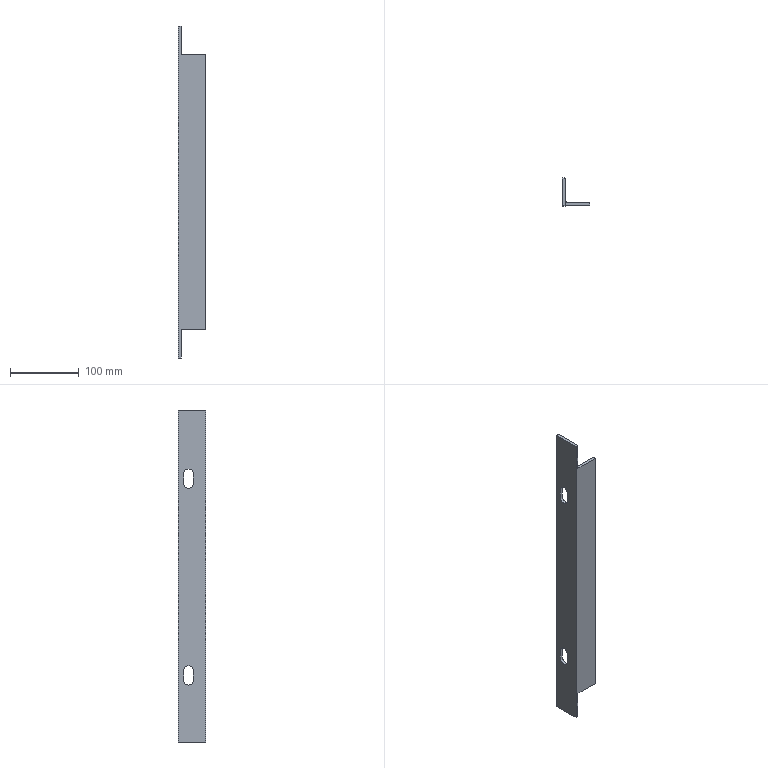Part | SolidWorks | features ICE 3, Fillet 2, ExtruThin 1, LPattern 1 | 1 solid | 23 faces | box 40 x 40 x 484.14 mm | volume 134390 mm3 | plane 14 | cylinder 9 | commonest cylinder face diameters 14 x6 2.667 x2 10 x1
STEP:
#1=CARTESIAN_POINT('',(0.,32.,90.));
#2=VERTEX_POINT('',#1);
#3=CARTESIAN_POINT('',(0.,25.,83.));
#4=VERTEX_POINT('',#3);
#5=CARTESIAN_POINT('',(0.,25.,90.));
#6=DIRECTION('',(-1.,0.,0.));
#7=DIRECTION('',(0.,0.,1.));
#8=AXIS2_PLACEMENT_3D('',#5,#6,#7);
#9=CIRCLE('',#8,7.);
#10=EDGE_CURVE('',#2,#4,#9,.T.);
#11=ORIENTED_EDGE('',*,*,#10,.T.);
#12=CARTESIAN_POINT('',(4.,25.,83.));
#13=VERTEX_POINT('',#12);
#14=CARTESIAN_POINT('',(-10.,25.,83.));
#15=DIRECTION('',(1.,0.,0.));
#16=VECTOR('',#15,1000.);
#17=LINE('',#14,#16);
#18=EDGE_CURVE('',#4,#13,#17,.T.);
#19=ORIENTED_EDGE('',*,*,#18,.T.);
#20=CARTESIAN_POINT('',(4.,32.,90.));
#21=VERTEX_POINT('',#20);
#22=CARTESIAN_POINT('',(4.,25.,90.));
#23=DIRECTION('',(1.,0.,0.));
#24=DIRECTION('',(0.,0.,-1.));
#25=AXIS2_PLACEMENT_3D('',#22,#23,#24);
#26=CIRCLE('',#25,7.);
#27=EDGE_CURVE('',#13,#21,#26,.T.);
#28=ORIENTED_EDGE('',*,*,#27,.T.);
#29=CARTESIAN_POINT('',(-10.,32.,90.));
#30=DIRECTION('',(1.,0.,0.));
#31=VECTOR('',#30,1000.);
#32=LINE('',#29,#31);
#33=EDGE_CURVE('',#2,#21,#32,.T.);
#34=ORIENTED_EDGE('',*,*,#33,.F.);
#35=EDGE_LOOP('',(#11,#19,#28,#34));
#36=FACE_OUTER_BOUND('',#35,.T.);
#37=CARTESIAN_POINT('',(-10.,25.,90.));
#38=DIRECTION('',(1.,0.,0.));
#39=DIRECTION('',(0.,0.,-1.));
#40=AXIS2_PLACEMENT_3D('',#37,#38,#39);
#41=CYLINDRICAL_SURFACE('',#40,7.);
#42=ADVANCED_FACE('',(#36),#41,.F.);
#43=CARTESIAN_POINT('',(0.,32.,377.14));
#44=VERTEX_POINT('',#43);
#45=CARTESIAN_POINT('',(0.,25.,370.14));
#46=VERTEX_POINT('',#45);
#47=CARTESIAN_POINT('',(0.,25.,377.14));
#48=DIRECTION('',(-1.,0.,0.));
#49=DIRECTION('',(0.,0.,1.));
#50=AXIS2_PLACEMENT_3D('',#47,#48,#49);
#51=CIRCLE('',#50,7.);
#52=EDGE_CURVE('',#44,#46,#51,.T.);
#53=ORIENTED_EDGE('',*,*,#52,.T.);
#54=CARTESIAN_POINT('',(4.,25.,370.14));
#55=VERTEX_POINT('',#54);
#56=CARTESIAN_POINT('',(-10.,25.,370.14));
#57=DIRECTION('',(1.,0.,0.));
#58=VECTOR('',#57,1000.);
#59=LINE('',#56,#58);
#60=EDGE_CURVE('',#46,#55,#59,.T.);
#61=ORIENTED_EDGE('',*,*,#60,.T.);
#62=CARTESIAN_POINT('',(4.,32.,377.14));
#63=VERTEX_POINT('',#62);
#64=CARTESIAN_POINT('',(4.,25.,377.14));
#65=DIRECTION('',(1.,0.,0.));
#66=DIRECTION('',(0.,0.,-1.));
#67=AXIS2_PLACEMENT_3D('',#64,#65,#66);
#68=CIRCLE('',#67,7.);
#69=EDGE_CURVE('',#55,#63,#68,.T.);
#70=ORIENTED_EDGE('',*,*,#69,.T.);
#71=CARTESIAN_POINT('',(-10.,32.,377.14));
#72=DIRECTION('',(1.,0.,0.));
#73=VECTOR('',#72,1000.);
#74=LINE('',#71,#73);
#75=EDGE_CURVE('',#44,#63,#74,.T.);
#76=ORIENTED_EDGE('',*,*,#75,.F.);
#77=EDGE_LOOP('',(#53,#61,#70,#76));
#78=FACE_OUTER_BOUND('',#77,.T.);
#79=CARTESIAN_POINT('',(-10.,25.,377.14));
#80=DIRECTION('',(1.,0.,0.));
#81=DIRECTION('',(0.,0.,-1.));
#82=AXIS2_PLACEMENT_3D('',#79,#80,#81);
#83=CYLINDRICAL_SURFACE('',#82,7.);
#84=ADVANCED_FACE('',(#78),#83,.F.);
#85=CARTESIAN_POINT('',(4.,18.,104.));
#86=VERTEX_POINT('',#85);
#87=CARTESIAN_POINT('',(4.,18.,90.));
#88=VERTEX_POINT('',#87);
#89=CARTESIAN_POINT('',(4.,18.,104.));
#90=DIRECTION('',(0.,0.,-1.));
#91=VECTOR('',#90,1000.);
#92=LINE('',#89,#91);
#93=EDGE_CURVE('',#86,#88,#92,.T.);
#94=ORIENTED_EDGE('',*,*,#93,.F.);
#95=CARTESIAN_POINT('',(4.,32.,104.));
#96=VERTEX_POINT('',#95);
#97=CARTESIAN_POINT('',(4.,25.,104.));
#98=DIRECTION('',(1.,0.,0.));
#99=DIRECTION('',(0.,0.,-1.));
#100=AXIS2_PLACEMENT_3D('',#97,#98,#99);
#101=CIRCLE('',#100,7.);
#102=EDGE_CURVE('',#96,#86,#101,.T.);
#103=ORIENTED_EDGE('',*,*,#102,.F.);
#104=CARTESIAN_POINT('',(4.,32.,104.));
#105=DIRECTION('',(0.,0.,1.));
#106=VECTOR('',#105,1000.);
#107=LINE('',#104,#106);
#108=EDGE_CURVE('',#21,#96,#107,.T.);
#109=ORIENTED_EDGE('',*,*,#108,.F.);
#110=ORIENTED_EDGE('',*,*,#27,.F.);
#111=CARTESIAN_POINT('',(4.,25.,90.));
#112=DIRECTION('',(1.,0.,0.));
#113=DIRECTION('',(0.,0.,-1.));
#114=AXIS2_PLACEMENT_3D('',#111,#112,#113);
#115=CIRCLE('',#114,7.);
#116=EDGE_CURVE('',#88,#13,#115,.T.);
#117=ORIENTED_EDGE('',*,*,#116,.F.);
#118=EDGE_LOOP('',(#94,#103,#109,#110,#117));
#119=FACE_BOUND('',#118,.T.);
#120=CARTESIAN_POINT('',(4.,18.,391.14));
#121=VERTEX_POINT('',#120);
#122=CARTESIAN_POINT('',(4.,18.,377.14));
#123=VERTEX_POINT('',#122);
#124=CARTESIAN_POINT('',(4.,18.,391.14));
#125=DIRECTION('',(0.,0.,-1.));
#126=VECTOR('',#125,1000.);
#127=LINE('',#124,#126);
#128=EDGE_CURVE('',#121,#123,#127,.T.);
#129=ORIENTED_EDGE('',*,*,#128,.F.);
#130=CARTESIAN_POINT('',(4.,32.,391.14));
#131=VERTEX_POINT('',#130);
#132=CARTESIAN_POINT('',(4.,25.,391.14));
#133=DIRECTION('',(1.,0.,0.));
#134=DIRECTION('',(0.,0.,-1.));
#135=AXIS2_PLACEMENT_3D('',#132,#133,#134);
#136=CIRCLE('',#135,7.);
#137=EDGE_CURVE('',#131,#121,#136,.T.);
#138=ORIENTED_EDGE('',*,*,#137,.F.);
#139=CARTESIAN_POINT('',(4.,32.,391.14));
#140=DIRECTION('',(0.,0.,1.));
#141=VECTOR('',#140,1000.);
#142=LINE('',#139,#141);
#143=EDGE_CURVE('',#63,#131,#142,.T.);
#144=ORIENTED_EDGE('',*,*,#143,.F.);
#145=ORIENTED_EDGE('',*,*,#69,.F.);
#146=CARTESIAN_POINT('',(4.,25.,377.14));
#147=DIRECTION('',(1.,0.,0.));
#148=DIRECTION('',(0.,0.,-1.));
#149=AXIS2_PLACEMENT_3D('',#146,#147,#148);
#150=CIRCLE('',#149,7.);
#151=EDGE_CURVE('',#123,#55,#150,.T.);
#152=ORIENTED_EDGE('',*,*,#151,.F.);
#153=EDGE_LOOP('',(#129,#138,#144,#145,#152));
#154=FACE_BOUND('',#153,.T.);
#155=CARTESIAN_POINT('',(4.,38.667,0.));
#156=VERTEX_POINT('',#155);
#157=CARTESIAN_POINT('',(4.,38.667,484.14));
#158=VERTEX_POINT('',#157);
#159=CARTESIAN_POINT('',(4.,38.667,484.14));
#160=DIRECTION('',(0.,0.,1.));
#161=VECTOR('',#160,1000.);
#162=LINE('',#159,#161);
#163=EDGE_CURVE('',#156,#158,#162,.T.);
#164=ORIENTED_EDGE('',*,*,#163,.T.);
#165=CARTESIAN_POINT('',(4.,0.,484.14));
#166=VERTEX_POINT('',#165);
#167=CARTESIAN_POINT('',(4.,0.,484.14));
#168=DIRECTION('',(0.,1.,0.));
#169=VECTOR('',#168,1000.);
#170=LINE('',#167,#169);
#171=EDGE_CURVE('',#166,#158,#170,.T.);
#172=ORIENTED_EDGE('',*,*,#171,.F.);
#173=CARTESIAN_POINT('',(4.,0.,443.14));
#174=VERTEX_POINT('',#173);
#175=CARTESIAN_POINT('',(4.,0.,484.14));
#176=DIRECTION('',(0.,0.,-1.));
#177=VECTOR('',#176,1000.);
#178=LINE('',#175,#177);
#179=EDGE_CURVE('',#166,#174,#178,.T.);
#180=ORIENTED_EDGE('',*,*,#179,.T.);
#181=CARTESIAN_POINT('',(4.,9.,443.14));
#182=VERTEX_POINT('',#181);
#183=CARTESIAN_POINT('',(4.,40.,443.14));
#184=DIRECTION('',(0.,-1.,0.));
#185=VECTOR('',#184,1000.);
#186=LINE('',#183,#185);
#187=EDGE_CURVE('',#182,#174,#186,.T.);
#188=ORIENTED_EDGE('',*,*,#187,.F.);
#189=CARTESIAN_POINT('',(4.,9.,41.));
#190=VERTEX_POINT('',#189);
#191=CARTESIAN_POINT('',(4.,9.,0.));
#192=DIRECTION('',(0.,0.,-1.));
#193=VECTOR('',#192,1000.);
#194=LINE('',#191,#193);
#195=EDGE_CURVE('',#182,#190,#194,.T.);
#196=ORIENTED_EDGE('',*,*,#195,.T.);
#197=CARTESIAN_POINT('',(4.,0.,41.));
#198=VERTEX_POINT('',#197);
#199=CARTESIAN_POINT('',(4.,40.,41.));
#200=DIRECTION('',(0.,-1.,0.));
#201=VECTOR('',#200,1000.);
#202=LINE('',#199,#201);
#203=EDGE_CURVE('',#190,#198,#202,.T.);
#204=ORIENTED_EDGE('',*,*,#203,.T.);
#205=CARTESIAN_POINT('',(4.,0.,0.));
#206=VERTEX_POINT('',#205);
#207=CARTESIAN_POINT('',(4.,0.,0.));
#208=DIRECTION('',(0.,0.,-1.));
#209=VECTOR('',#208,1000.);
#210=LINE('',#207,#209);
#211=EDGE_CURVE('',#198,#206,#210,.T.);
#212=ORIENTED_EDGE('',*,*,#211,.T.);
#213=CARTESIAN_POINT('',(4.,0.,0.));
#214=DIRECTION('',(0.,1.,0.));
#215=VECTOR('',#214,1000.);
#216=LINE('',#213,#215);
#217=EDGE_CURVE('',#206,#156,#216,.T.);
#218=ORIENTED_EDGE('',*,*,#217,.T.);
#219=EDGE_LOOP('',(#164,#172,#180,#188,#196,#204,#212,#218));
#220=FACE_OUTER_BOUND('',#219,.T.);
#221=CARTESIAN_POINT('',(4.,0.,484.14));
#222=DIRECTION('',(-1.,0.,0.));
#223=DIRECTION('',(0.,0.,1.));
#224=AXIS2_PLACEMENT_3D('',#221,#222,#223);
#225=PLANE('',#224);
#226=ADVANCED_FACE('',(#119,#154,#220),#225,.F.);
#227=CARTESIAN_POINT('',(0.,40.,484.14));
#228=VERTEX_POINT('',#227);
#229=CARTESIAN_POINT('',(2.667,40.,484.14));
#230=VERTEX_POINT('',#229);
#231=CARTESIAN_POINT('',(0.,40.,484.14));
#232=DIRECTION('',(1.,0.,0.));
#233=VECTOR('',#232,1000.);
#234=LINE('',#231,#233);
#235=EDGE_CURVE('',#228,#230,#234,.T.);
#236=ORIENTED_EDGE('',*,*,#235,.T.);
#237=CARTESIAN_POINT('',(2.667,40.,0.));
#238=VERTEX_POINT('',#237);
#239=CARTESIAN_POINT('',(2.667,40.,0.));
#240=DIRECTION('',(0.,0.,-1.));
#241=VECTOR('',#240,1000.);
#242=LINE('',#239,#241);
#243=EDGE_CURVE('',#230,#238,#242,.T.);
#244=ORIENTED_EDGE('',*,*,#243,.T.);
#245=CARTESIAN_POINT('',(0.,40.,0.));
#246=VERTEX_POINT('',#245);
#247=CARTESIAN_POINT('',(0.,40.,0.));
#248=DIRECTION('',(1.,0.,0.));
#249=VECTOR('',#248,1000.);
#250=LINE('',#247,#249);
#251=EDGE_CURVE('',#246,#238,#250,.T.);
#252=ORIENTED_EDGE('',*,*,#251,.F.);
#253=CARTESIAN_POINT('',(0.,40.,484.14));
#254=DIRECTION('',(0.,0.,-1.));
#255=VECTOR('',#254,1000.);
#256=LINE('',#253,#255);
#257=EDGE_CURVE('',#228,#246,#256,.T.);
#258=ORIENTED_EDGE('',*,*,#257,.F.);
#259=EDGE_LOOP('',(#236,#244,#252,#258));
#260=FACE_OUTER_BOUND('',#259,.T.);
#261=CARTESIAN_POINT('',(0.,40.,484.14));
#262=DIRECTION('',(0.,1.,0.));
#263=DIRECTION('',(0.,0.,1.));
#264=AXIS2_PLACEMENT_3D('',#261,#262,#263);
#265=PLANE('',#264);
#266=ADVANCED_FACE('',(#260),#265,.T.);
#267=CARTESIAN_POINT('',(0.,18.,104.));
#268=VERTEX_POINT('',#267);
#269=CARTESIAN_POINT('',(0.,32.,104.));
#270=VERTEX_POINT('',#269);
#271=CARTESIAN_POINT('',(0.,25.,104.));
#272=DIRECTION('',(-1.,0.,0.));
#273=DIRECTION('',(0.,0.,1.));
#274=AXIS2_PLACEMENT_3D('',#271,#272,#273);
#275=CIRCLE('',#274,7.);
#276=EDGE_CURVE('',#268,#270,#275,.T.);
#277=ORIENTED_EDGE('',*,*,#276,.F.);
#278=CARTESIAN_POINT('',(0.,18.,90.));
#279=VERTEX_POINT('',#278);
#280=CARTESIAN_POINT('',(0.,18.,484.14));
#281=DIRECTION('',(0.,0.,1.));
#282=VECTOR('',#281,1000.);
#283=LINE('',#280,#282);
#284=EDGE_CURVE('',#279,#268,#283,.T.);
#285=ORIENTED_EDGE('',*,*,#284,.F.);
#286=CARTESIAN_POINT('',(0.,25.,90.));
#287=DIRECTION('',(-1.,0.,0.));
#288=DIRECTION('',(0.,0.,1.));
#289=AXIS2_PLACEMENT_3D('',#286,#287,#288);
#290=CIRCLE('',#289,7.);
#291=EDGE_CURVE('',#4,#279,#290,.T.);
#292=ORIENTED_EDGE('',*,*,#291,.F.);
#293=ORIENTED_EDGE('',*,*,#10,.F.);
#294=CARTESIAN_POINT('',(0.,32.,484.14));
#295=DIRECTION('',(0.,0.,-1.));
#296=VECTOR('',#295,1000.);
#297=LINE('',#294,#296);
#298=EDGE_CURVE('',#270,#2,#297,.T.);
#299=ORIENTED_EDGE('',*,*,#298,.F.);
#300=EDGE_LOOP('',(#277,#285,#292,#293,#299));
#301=FACE_BOUND('',#300,.T.);
#302=CARTESIAN_POINT('',(0.,18.,391.14));
#303=VERTEX_POINT('',#302);
#304=CARTESIAN_POINT('',(0.,32.,391.14));
#305=VERTEX_POINT('',#304);
#306=CARTESIAN_POINT('',(0.,25.,391.14));
#307=DIRECTION('',(-1.,0.,0.));
#308=DIRECTION('',(0.,0.,1.));
#309=AXIS2_PLACEMENT_3D('',#306,#307,#308);
#310=CIRCLE('',#309,7.);
#311=EDGE_CURVE('',#303,#305,#310,.T.);
#312=ORIENTED_EDGE('',*,*,#311,.F.);
#313=CARTESIAN_POINT('',(0.,18.,377.14));
#314=VERTEX_POINT('',#313);
#315=CARTESIAN_POINT('',(0.,18.,484.14));
#316=DIRECTION('',(0.,0.,1.));
#317=VECTOR('',#316,1000.);
#318=LINE('',#315,#317);
#319=EDGE_CURVE('',#314,#303,#318,.T.);
#320=ORIENTED_EDGE('',*,*,#319,.F.);
#321=CARTESIAN_POINT('',(0.,25.,377.14));
#322=DIRECTION('',(-1.,0.,0.));
#323=DIRECTION('',(0.,0.,1.));
#324=AXIS2_PLACEMENT_3D('',#321,#322,#323);
#325=CIRCLE('',#324,7.);
#326=EDGE_CURVE('',#46,#314,#325,.T.);
#327=ORIENTED_EDGE('',*,*,#326,.F.);
#328=ORIENTED_EDGE('',*,*,#52,.F.);
#329=CARTESIAN_POINT('',(0.,32.,484.14));
#330=DIRECTION('',(0.,0.,-1.));
#331=VECTOR('',#330,1000.);
#332=LINE('',#329,#331);
#333=EDGE_CURVE('',#305,#44,#332,.T.);
#334=ORIENTED_EDGE('',*,*,#333,.F.);
#335=EDGE_LOOP('',(#312,#320,#327,#328,#334));
#336=FACE_BOUND('',#335,.T.);
#337=CARTESIAN_POINT('',(0.,0.,0.));
#338=VERTEX_POINT('',#337);
#339=CARTESIAN_POINT('',(0.,0.,0.));
#340=DIRECTION('',(0.,1.,0.));
#341=VECTOR('',#340,1000.);
#342=LINE('',#339,#341);
#343=EDGE_CURVE('',#338,#246,#342,.T.);
#344=ORIENTED_EDGE('',*,*,#343,.F.);
#345=CARTESIAN_POINT('',(0.,0.,484.14));
#346=VERTEX_POINT('',#345);
#347=CARTESIAN_POINT('',(0.,0.,484.14));
#348=DIRECTION('',(0.,0.,-1.));
#349=VECTOR('',#348,1000.);
#350=LINE('',#347,#349);
#351=EDGE_CURVE('',#346,#338,#350,.T.);
#352=ORIENTED_EDGE('',*,*,#351,.F.);
#353=CARTESIAN_POINT('',(0.,0.,484.14));
#354=DIRECTION('',(0.,1.,0.));
#355=VECTOR('',#354,1000.);
#356=LINE('',#353,#355);
#357=EDGE_CURVE('',#346,#228,#356,.T.);
#358=ORIENTED_EDGE('',*,*,#357,.T.);
#359=ORIENTED_EDGE('',*,*,#257,.T.);
#360=EDGE_LOOP('',(#344,#352,#358,#359));
#361=FACE_OUTER_BOUND('',#360,.T.);
#362=CARTESIAN_POINT('',(0.,0.,484.14));
#363=DIRECTION('',(-1.,0.,0.));
#364=DIRECTION('',(0.,0.,1.));
#365=AXIS2_PLACEMENT_3D('',#362,#363,#364);
#366=PLANE('',#365);
#367=ADVANCED_FACE('',(#301,#336,#361),#366,.T.);
#368=ORIENTED_EDGE('',*,*,#179,.F.);
#369=CARTESIAN_POINT('',(0.,0.,484.14));
#370=DIRECTION('',(-1.,0.,0.));
#371=VECTOR('',#370,1000.);
#372=LINE('',#369,#371);
#373=EDGE_CURVE('',#166,#346,#372,.T.);
#374=ORIENTED_EDGE('',*,*,#373,.T.);
#375=ORIENTED_EDGE('',*,*,#351,.T.);
#376=CARTESIAN_POINT('',(0.,0.,0.));
#377=DIRECTION('',(-1.,0.,0.));
#378=VECTOR('',#377,1000.);
#379=LINE('',#376,#378);
#380=EDGE_CURVE('',#206,#338,#379,.T.);
#381=ORIENTED_EDGE('',*,*,#380,.F.);
#382=ORIENTED_EDGE('',*,*,#211,.F.);
#383=CARTESIAN_POINT('',(40.,0.,41.));
#384=VERTEX_POINT('',#383);
#385=CARTESIAN_POINT('',(40.,0.,41.));
#386=DIRECTION('',(-1.,0.,0.));
#387=VECTOR('',#386,1000.);
#388=LINE('',#385,#387);
#389=EDGE_CURVE('',#384,#198,#388,.T.);
#390=ORIENTED_EDGE('',*,*,#389,.F.);
#391=CARTESIAN_POINT('',(40.,0.,443.14));
#392=VERTEX_POINT('',#391);
#393=CARTESIAN_POINT('',(40.,0.,484.14));
#394=DIRECTION('',(0.,0.,-1.));
#395=VECTOR('',#394,1000.);
#396=LINE('',#393,#395);
#397=EDGE_CURVE('',#392,#384,#396,.T.);
#398=ORIENTED_EDGE('',*,*,#397,.F.);
#399=CARTESIAN_POINT('',(4.,0.,443.14));
#400=DIRECTION('',(1.,0.,0.));
#401=VECTOR('',#400,1000.);
#402=LINE('',#399,#401);
#403=EDGE_CURVE('',#174,#392,#402,.T.);
#404=ORIENTED_EDGE('',*,*,#403,.F.);
#405=EDGE_LOOP('',(#368,#374,#375,#381,#382,#390,#398,#404));
#406=FACE_OUTER_BOUND('',#405,.T.);
#407=CARTESIAN_POINT('',(0.,0.,484.14));
#408=DIRECTION('',(0.,-1.,0.));
#409=DIRECTION('',(0.,0.,-1.));
#410=AXIS2_PLACEMENT_3D('',#407,#408,#409);
#411=PLANE('',#410);
#412=ADVANCED_FACE('',(#406),#411,.T.);
#413=CARTESIAN_POINT('',(40.,2.667,443.14));
#414=VERTEX_POINT('',#413);
#415=CARTESIAN_POINT('',(40.,40.,443.14));
#416=DIRECTION('',(0.,-1.,0.));
#417=VECTOR('',#416,1000.);
#418=LINE('',#415,#417);
#419=EDGE_CURVE('',#414,#392,#418,.T.);
#420=ORIENTED_EDGE('',*,*,#419,.T.);
#421=ORIENTED_EDGE('',*,*,#397,.T.);
#422=CARTESIAN_POINT('',(40.,2.667,41.));
#423=VERTEX_POINT('',#422);
#424=CARTESIAN_POINT('',(40.,40.,41.));
#425=DIRECTION('',(0.,-1.,0.));
#426=VECTOR('',#425,1000.);
#427=LINE('',#424,#426);
#428=EDGE_CURVE('',#423,#384,#427,.T.);
#429=ORIENTED_EDGE('',*,*,#428,.F.);
#430=CARTESIAN_POINT('',(40.,2.667,484.14));
#431=DIRECTION('',(0.,0.,1.));
#432=VECTOR('',#431,1000.);
#433=LINE('',#430,#432);
#434=EDGE_CURVE('',#423,#414,#433,.T.);
#435=ORIENTED_EDGE('',*,*,#434,.T.);
#436=EDGE_LOOP('',(#420,#421,#429,#435));
#437=FACE_OUTER_BOUND('',#436,.T.);
#438=CARTESIAN_POINT('',(40.,4.,484.14));
#439=DIRECTION('',(1.,0.,0.));
#440=DIRECTION('',(0.,0.,-1.));
#441=AXIS2_PLACEMENT_3D('',#438,#439,#440);
#442=PLANE('',#441);
#443=ADVANCED_FACE('',(#437),#442,.T.);
#444=CARTESIAN_POINT('',(9.,4.,41.));
#445=VERTEX_POINT('',#444);
#446=CARTESIAN_POINT('',(9.,4.,443.14));
#447=VERTEX_POINT('',#446);
#448=CARTESIAN_POINT('',(9.,4.,484.14));
#449=DIRECTION('',(0.,0.,1.));
#450=VECTOR('',#449,1000.);
#451=LINE('',#448,#450);
#452=EDGE_CURVE('',#445,#447,#451,.T.);
#453=ORIENTED_EDGE('',*,*,#452,.T.);
#454=CARTESIAN_POINT('',(38.667,4.,443.14));
#455=VERTEX_POINT('',#454);
#456=CARTESIAN_POINT('',(0.,4.,443.14));
#457=DIRECTION('',(1.,0.,0.));
#458=VECTOR('',#457,1000.);
#459=LINE('',#456,#458);
#460=EDGE_CURVE('',#447,#455,#459,.T.);
#461=ORIENTED_EDGE('',*,*,#460,.T.);
#462=CARTESIAN_POINT('',(38.667,4.,41.));
#463=VERTEX_POINT('',#462);
#464=CARTESIAN_POINT('',(38.667,4.,0.));
#465=DIRECTION('',(0.,0.,-1.));
#466=VECTOR('',#465,1000.);
#467=LINE('',#464,#466);
#468=EDGE_CURVE('',#455,#463,#467,.T.);
#469=ORIENTED_EDGE('',*,*,#468,.T.);
#470=CARTESIAN_POINT('',(0.,4.,41.));
#471=DIRECTION('',(-1.,0.,0.));
#472=VECTOR('',#471,1000.);
#473=LINE('',#470,#472);
#474=EDGE_CURVE('',#463,#445,#473,.T.);
#475=ORIENTED_EDGE('',*,*,#474,.T.);
#476=EDGE_LOOP('',(#453,#461,#469,#475));
#477=FACE_OUTER_BOUND('',#476,.T.);
#478=CARTESIAN_POINT('',(0.,4.,484.14));
#479=DIRECTION('',(0.,-1.,0.));
#480=DIRECTION('',(0.,0.,-1.));
#481=AXIS2_PLACEMENT_3D('',#478,#479,#480);
#482=PLANE('',#481);
#483=ADVANCED_FACE('',(#477),#482,.F.);
#484=ORIENTED_EDGE('',*,*,#373,.F.);
#485=ORIENTED_EDGE('',*,*,#171,.T.);
#486=CARTESIAN_POINT('',(2.667,38.667,484.14));
#487=DIRECTION('',(0.,0.,1.));
#488=DIRECTION('',(-1.,0.,0.));
#489=AXIS2_PLACEMENT_3D('',#486,#487,#488);
#490=CIRCLE('',#489,1.333);
#491=EDGE_CURVE('',#158,#230,#490,.T.);
#492=ORIENTED_EDGE('',*,*,#491,.T.);
#493=ORIENTED_EDGE('',*,*,#235,.F.);
#494=ORIENTED_EDGE('',*,*,#357,.F.);
#495=EDGE_LOOP('',(#484,#485,#492,#493,#494));
#496=FACE_OUTER_BOUND('',#495,.T.);
#497=CARTESIAN_POINT('',(0.,0.,484.14));
#498=DIRECTION('',(0.,0.,-1.));
#499=DIRECTION('',(-1.,0.,0.));
#500=AXIS2_PLACEMENT_3D('',#497,#498,#499);
#501=PLANE('',#500);
#502=ADVANCED_FACE('',(#496),#501,.F.);
#503=ORIENTED_EDGE('',*,*,#217,.F.);
#504=ORIENTED_EDGE('',*,*,#380,.T.);
#505=ORIENTED_EDGE('',*,*,#343,.T.);
#506=ORIENTED_EDGE('',*,*,#251,.T.);
#507=CARTESIAN_POINT('',(2.667,38.667,0.));
#508=DIRECTION('',(0.,0.,-1.));
#509=DIRECTION('',(-1.,0.,0.));
#510=AXIS2_PLACEMENT_3D('',#507,#508,#509);
#511=CIRCLE('',#510,1.333);
#512=EDGE_CURVE('',#238,#156,#511,.T.);
#513=ORIENTED_EDGE('',*,*,#512,.T.);
#514=EDGE_LOOP('',(#503,#504,#505,#506,#513));
#515=FACE_OUTER_BOUND('',#514,.T.);
#516=CARTESIAN_POINT('',(0.,0.,0.));
#517=DIRECTION('',(0.,0.,-1.));
#518=DIRECTION('',(-1.,0.,0.));
#519=AXIS2_PLACEMENT_3D('',#516,#517,#518);
#520=PLANE('',#519);
#521=ADVANCED_FACE('',(#515),#520,.T.);
#522=ORIENTED_EDGE('',*,*,#195,.F.);
#523=CARTESIAN_POINT('',(9.,9.,443.14));
#524=DIRECTION('',(0.,0.,1.));
#525=DIRECTION('',(-1.,0.,0.));
#526=AXIS2_PLACEMENT_3D('',#523,#524,#525);
#527=CIRCLE('',#526,5.);
#528=EDGE_CURVE('',#182,#447,#527,.T.);
#529=ORIENTED_EDGE('',*,*,#528,.T.);
#530=ORIENTED_EDGE('',*,*,#452,.F.);
#531=CARTESIAN_POINT('',(9.,9.,41.));
#532=DIRECTION('',(0.,0.,-1.));
#533=DIRECTION('',(1.,0.,0.));
#534=AXIS2_PLACEMENT_3D('',#531,#532,#533);
#535=CIRCLE('',#534,5.);
#536=EDGE_CURVE('',#445,#190,#535,.T.);
#537=ORIENTED_EDGE('',*,*,#536,.T.);
#538=EDGE_LOOP('',(#522,#529,#530,#537));
#539=FACE_OUTER_BOUND('',#538,.T.);
#540=CARTESIAN_POINT('',(9.,9.,484.14));
#541=DIRECTION('',(0.,0.,1.));
#542=DIRECTION('',(1.,0.,0.));
#543=AXIS2_PLACEMENT_3D('',#540,#541,#542);
#544=CYLINDRICAL_SURFACE('',#543,5.);
#545=ADVANCED_FACE('',(#539),#544,.F.);
#546=CARTESIAN_POINT('',(38.667,2.667,443.14));
#547=DIRECTION('',(0.,0.,1.));
#548=DIRECTION('',(-1.,0.,0.));
#549=AXIS2_PLACEMENT_3D('',#546,#547,#548);
#550=CIRCLE('',#549,1.333);
#551=EDGE_CURVE('',#414,#455,#550,.T.);
#552=ORIENTED_EDGE('',*,*,#551,.F.);
#553=ORIENTED_EDGE('',*,*,#434,.F.);
#554=CARTESIAN_POINT('',(38.667,2.667,41.));
#555=DIRECTION('',(0.,0.,-1.));
#556=DIRECTION('',(1.,0.,0.));
#557=AXIS2_PLACEMENT_3D('',#554,#555,#556);
#558=CIRCLE('',#557,1.333);
#559=EDGE_CURVE('',#463,#423,#558,.T.);
#560=ORIENTED_EDGE('',*,*,#559,.F.);
#561=ORIENTED_EDGE('',*,*,#468,.F.);
#562=EDGE_LOOP('',(#552,#553,#560,#561));
#563=FACE_OUTER_BOUND('',#562,.T.);
#564=CARTESIAN_POINT('',(38.667,2.667,484.14));
#565=DIRECTION('',(0.,0.,1.));
#566=DIRECTION('',(1.,0.,0.));
#567=AXIS2_PLACEMENT_3D('',#564,#565,#566);
#568=CYLINDRICAL_SURFACE('',#567,1.333);
#569=ADVANCED_FACE('',(#563),#568,.T.);
#570=ORIENTED_EDGE('',*,*,#491,.F.);
#571=ORIENTED_EDGE('',*,*,#163,.F.);
#572=ORIENTED_EDGE('',*,*,#512,.F.);
#573=ORIENTED_EDGE('',*,*,#243,.F.);
#574=EDGE_LOOP('',(#570,#571,#572,#573));
#575=FACE_OUTER_BOUND('',#574,.T.);
#576=CARTESIAN_POINT('',(2.667,38.667,484.14));
#577=DIRECTION('',(0.,0.,1.));
#578=DIRECTION('',(1.,0.,0.));
#579=AXIS2_PLACEMENT_3D('',#576,#577,#578);
#580=CYLINDRICAL_SURFACE('',#579,1.333);
#581=ADVANCED_FACE('',(#575),#580,.T.);
#582=ORIENTED_EDGE('',*,*,#474,.F.);
#583=ORIENTED_EDGE('',*,*,#559,.T.);
#584=ORIENTED_EDGE('',*,*,#428,.T.);
#585=ORIENTED_EDGE('',*,*,#389,.T.);
#586=ORIENTED_EDGE('',*,*,#203,.F.);
#587=ORIENTED_EDGE('',*,*,#536,.F.);
#588=EDGE_LOOP('',(#582,#583,#584,#585,#586,#587));
#589=FACE_OUTER_BOUND('',#588,.T.);
#590=CARTESIAN_POINT('',(40.,40.,41.));
#591=DIRECTION('',(0.,0.,1.));
#592=DIRECTION('',(1.,0.,0.));
#593=AXIS2_PLACEMENT_3D('',#590,#591,#592);
#594=PLANE('',#593);
#595=ADVANCED_FACE('',(#589),#594,.F.);
#596=ORIENTED_EDGE('',*,*,#187,.T.);
#597=ORIENTED_EDGE('',*,*,#403,.T.);
#598=ORIENTED_EDGE('',*,*,#419,.F.);
#599=ORIENTED_EDGE('',*,*,#551,.T.);
#600=ORIENTED_EDGE('',*,*,#460,.F.);
#601=ORIENTED_EDGE('',*,*,#528,.F.);
#602=EDGE_LOOP('',(#596,#597,#598,#599,#600,#601));
#603=FACE_OUTER_BOUND('',#602,.T.);
#604=CARTESIAN_POINT('',(4.,40.,443.14));
#605=DIRECTION('',(0.,0.,-1.));
#606=DIRECTION('',(-1.,0.,0.));
#607=AXIS2_PLACEMENT_3D('',#604,#605,#606);
#608=PLANE('',#607);
#609=ADVANCED_FACE('',(#603),#608,.F.);
#610=ORIENTED_EDGE('',*,*,#311,.T.);
#611=CARTESIAN_POINT('',(-10.,32.,391.14));
#612=DIRECTION('',(1.,0.,0.));
#613=VECTOR('',#612,1000.);
#614=LINE('',#611,#613);
#615=EDGE_CURVE('',#305,#131,#614,.T.);
#616=ORIENTED_EDGE('',*,*,#615,.T.);
#617=ORIENTED_EDGE('',*,*,#137,.T.);
#618=CARTESIAN_POINT('',(-10.,18.,391.14));
#619=DIRECTION('',(1.,0.,0.));
#620=VECTOR('',#619,1000.);
#621=LINE('',#618,#620);
#622=EDGE_CURVE('',#303,#121,#621,.T.);
#623=ORIENTED_EDGE('',*,*,#622,.F.);
#624=EDGE_LOOP('',(#610,#616,#617,#623));
#625=FACE_OUTER_BOUND('',#624,.T.);
#626=CARTESIAN_POINT('',(-10.,25.,391.14));
#627=DIRECTION('',(1.,0.,0.));
#628=DIRECTION('',(0.,0.,-1.));
#629=AXIS2_PLACEMENT_3D('',#626,#627,#628);
#630=CYLINDRICAL_SURFACE('',#629,7.);
#631=ADVANCED_FACE('',(#625),#630,.F.);
#632=ORIENTED_EDGE('',*,*,#333,.T.);
#633=ORIENTED_EDGE('',*,*,#75,.T.);
#634=ORIENTED_EDGE('',*,*,#143,.T.);
#635=ORIENTED_EDGE('',*,*,#615,.F.);
#636=EDGE_LOOP('',(#632,#633,#634,#635));
#637=FACE_OUTER_BOUND('',#636,.T.);
#638=CARTESIAN_POINT('',(-10.,32.,391.14));
#639=DIRECTION('',(0.,1.,0.));
#640=DIRECTION('',(0.,0.,1.));
#641=AXIS2_PLACEMENT_3D('',#638,#639,#640);
#642=PLANE('',#641);
#643=ADVANCED_FACE('',(#637),#642,.F.);
#644=ORIENTED_EDGE('',*,*,#60,.F.);
#645=ORIENTED_EDGE('',*,*,#326,.T.);
#646=CARTESIAN_POINT('',(-10.,18.,377.14));
#647=DIRECTION('',(1.,0.,0.));
#648=VECTOR('',#647,1000.);
#649=LINE('',#646,#648);
#650=EDGE_CURVE('',#314,#123,#649,.T.);
#651=ORIENTED_EDGE('',*,*,#650,.T.);
#652=ORIENTED_EDGE('',*,*,#151,.T.);
#653=EDGE_LOOP('',(#644,#645,#651,#652));
#654=FACE_OUTER_BOUND('',#653,.T.);
#655=CARTESIAN_POINT('',(-10.,25.,377.14));
#656=DIRECTION('',(1.,0.,0.));
#657=DIRECTION('',(0.,0.,-1.));
#658=AXIS2_PLACEMENT_3D('',#655,#656,#657);
#659=CYLINDRICAL_SURFACE('',#658,7.);
#660=ADVANCED_FACE('',(#654),#659,.F.);
#661=ORIENTED_EDGE('',*,*,#319,.T.);
#662=ORIENTED_EDGE('',*,*,#622,.T.);
#663=ORIENTED_EDGE('',*,*,#128,.T.);
#664=ORIENTED_EDGE('',*,*,#650,.F.);
#665=EDGE_LOOP('',(#661,#662,#663,#664));
#666=FACE_OUTER_BOUND('',#665,.T.);
#667=CARTESIAN_POINT('',(-10.,18.,391.14));
#668=DIRECTION('',(0.,-1.,0.));
#669=DIRECTION('',(0.,0.,-1.));
#670=AXIS2_PLACEMENT_3D('',#667,#668,#669);
#671=PLANE('',#670);
#672=ADVANCED_FACE('',(#666),#671,.F.);
#673=ORIENTED_EDGE('',*,*,#276,.T.);
#674=CARTESIAN_POINT('',(-10.,32.,104.));
#675=DIRECTION('',(1.,0.,0.));
#676=VECTOR('',#675,1000.);
#677=LINE('',#674,#676);
#678=EDGE_CURVE('',#270,#96,#677,.T.);
#679=ORIENTED_EDGE('',*,*,#678,.T.);
#680=ORIENTED_EDGE('',*,*,#102,.T.);
#681=CARTESIAN_POINT('',(-10.,18.,104.));
#682=DIRECTION('',(1.,0.,0.));
#683=VECTOR('',#682,1000.);
#684=LINE('',#681,#683);
#685=EDGE_CURVE('',#268,#86,#684,.T.);
#686=ORIENTED_EDGE('',*,*,#685,.F.);
#687=EDGE_LOOP('',(#673,#679,#680,#686));
#688=FACE_OUTER_BOUND('',#687,.T.);
#689=CARTESIAN_POINT('',(-10.,25.,104.));
#690=DIRECTION('',(1.,0.,0.));
#691=DIRECTION('',(0.,0.,-1.));
#692=AXIS2_PLACEMENT_3D('',#689,#690,#691);
#693=CYLINDRICAL_SURFACE('',#692,7.);
#694=ADVANCED_FACE('',(#688),#693,.F.);
#695=ORIENTED_EDGE('',*,*,#298,.T.);
#696=ORIENTED_EDGE('',*,*,#33,.T.);
#697=ORIENTED_EDGE('',*,*,#108,.T.);
#698=ORIENTED_EDGE('',*,*,#678,.F.);
#699=EDGE_LOOP('',(#695,#696,#697,#698));
#700=FACE_OUTER_BOUND('',#699,.T.);
#701=CARTESIAN_POINT('',(-10.,32.,104.));
#702=DIRECTION('',(0.,1.,0.));
#703=DIRECTION('',(0.,0.,1.));
#704=AXIS2_PLACEMENT_3D('',#701,#702,#703);
#705=PLANE('',#704);
#706=ADVANCED_FACE('',(#700),#705,.F.);
#707=ORIENTED_EDGE('',*,*,#18,.F.);
#708=ORIENTED_EDGE('',*,*,#291,.T.);
#709=CARTESIAN_POINT('',(-10.,18.,90.));
#710=DIRECTION('',(1.,0.,0.));
#711=VECTOR('',#710,1000.);
#712=LINE('',#709,#711);
#713=EDGE_CURVE('',#279,#88,#712,.T.);
#714=ORIENTED_EDGE('',*,*,#713,.T.);
#715=ORIENTED_EDGE('',*,*,#116,.T.);
#716=EDGE_LOOP('',(#707,#708,#714,#715));
#717=FACE_OUTER_BOUND('',#716,.T.);
#718=CARTESIAN_POINT('',(-10.,25.,90.));
#719=DIRECTION('',(1.,0.,0.));
#720=DIRECTION('',(0.,0.,-1.));
#721=AXIS2_PLACEMENT_3D('',#718,#719,#720);
#722=CYLINDRICAL_SURFACE('',#721,7.);
#723=ADVANCED_FACE('',(#717),#722,.F.);
#724=ORIENTED_EDGE('',*,*,#284,.T.);
#725=ORIENTED_EDGE('',*,*,#685,.T.);
#726=ORIENTED_EDGE('',*,*,#93,.T.);
#727=ORIENTED_EDGE('',*,*,#713,.F.);
#728=EDGE_LOOP('',(#724,#725,#726,#727));
#729=FACE_OUTER_BOUND('',#728,.T.);
#730=CARTESIAN_POINT('',(-10.,18.,104.));
#731=DIRECTION('',(0.,-1.,0.));
#732=DIRECTION('',(0.,0.,-1.));
#733=AXIS2_PLACEMENT_3D('',#730,#731,#732);
#734=PLANE('',#733);
#735=ADVANCED_FACE('',(#729),#734,.F.);
#736=CLOSED_SHELL('',(#42,#84,#226,#266,#367,#412,#443,#483,#502,#521,#545,#569,#581,#595,#609,#631,#643,#660,#672,#694,#706,#723,#735));
#737=MANIFOLD_SOLID_BREP('',#736);
#738=CARTESIAN_POINT('',(0.,0.,0.));
#739=DIRECTION('',(0.,0.,1.));
#740=DIRECTION('',(1.,0.,0.));
#741=AXIS2_PLACEMENT_3D('',#738,#739,#740);
#742=(LENGTH_UNIT()NAMED_UNIT(*)SI_UNIT(.MILLI.,.METRE.));
#743=UNCERTAINTY_MEASURE_WITH_UNIT(LENGTH_MEASURE(0.00001),#742,'','');
#744=(NAMED_UNIT(*)PLANE_ANGLE_UNIT()SI_UNIT($,.RADIAN.));
#745=(NAMED_UNIT(*)SI_UNIT($,.STERADIAN.)SOLID_ANGLE_UNIT());
#746=(GEOMETRIC_REPRESENTATION_CONTEXT(3)GLOBAL_UNCERTAINTY_ASSIGNED_CONTEXT((#743))GLOBAL_UNIT_ASSIGNED_CONTEXT((#742,#744,#745))REPRESENTATION_CONTEXT('',''));
#747=ADVANCED_BREP_SHAPE_REPRESENTATION('',(#737,#741),#746);